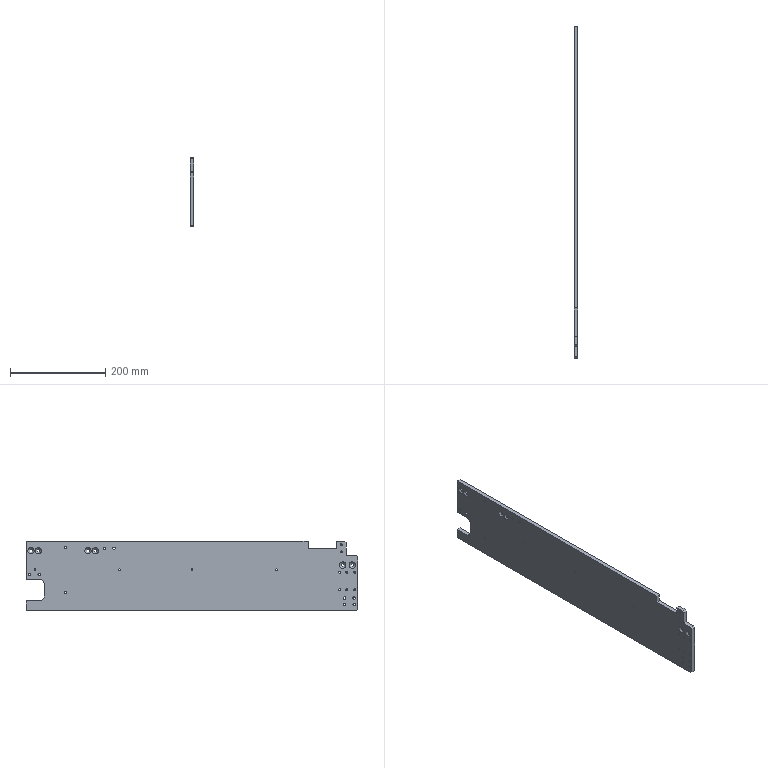Part | NX | features 5003_204_Mounting plate  2 | 1 solid | 55 faces | box 8 x 698 x 146 mm | volume 783248 mm3 | cylinder 30 | plane 19 | cone 6 | commonest cylinder face diameters 5 x10 4.2 x8 6.6 x6 3.3 x4 20 x2